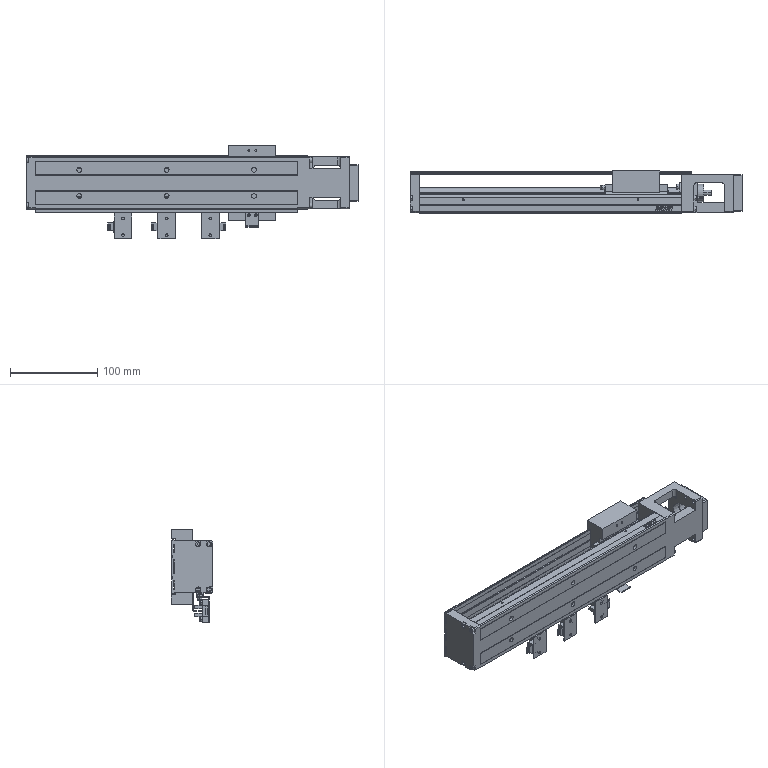Part | SolidWorks | 7 solids | 1654 faces | box 380 x 48 x 106.85 mm | volume 542226 mm3 | plane 979 | cylinder 417 | spline 146 | cone 110 | torus 2 | commonest cylinder face diameters 1 x80 5.5 x68 3 x58 6 x45 9.5 x20 2.113 x16